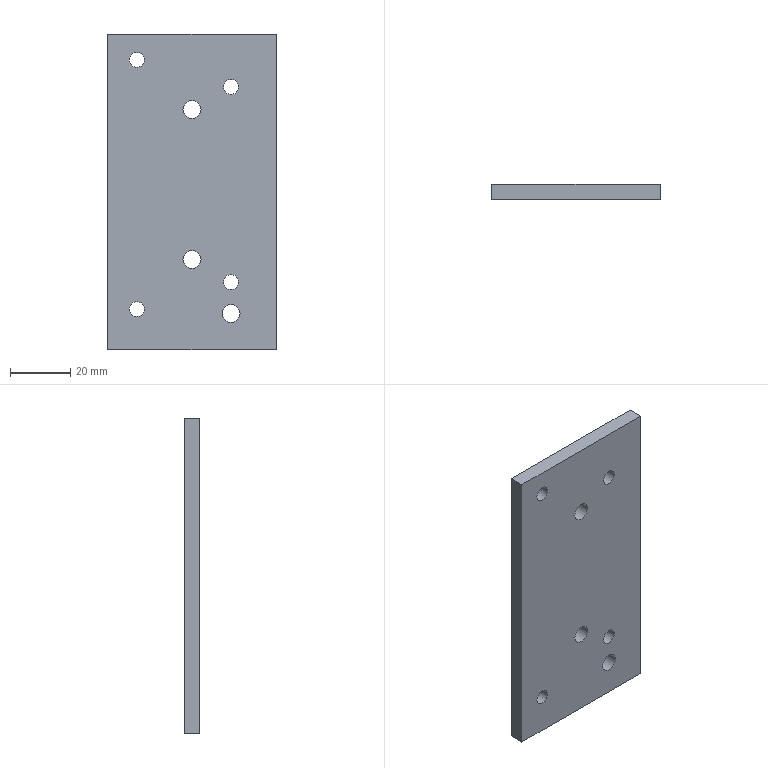Part | STEP file | spacer plate 4 | 1 solid | 20 faces | box 56 x 5 x 105 mm | volume 28583 mm3 | cylinder 14 | plane 6 | commonest cylinder face diameters 5 x8 6 x6